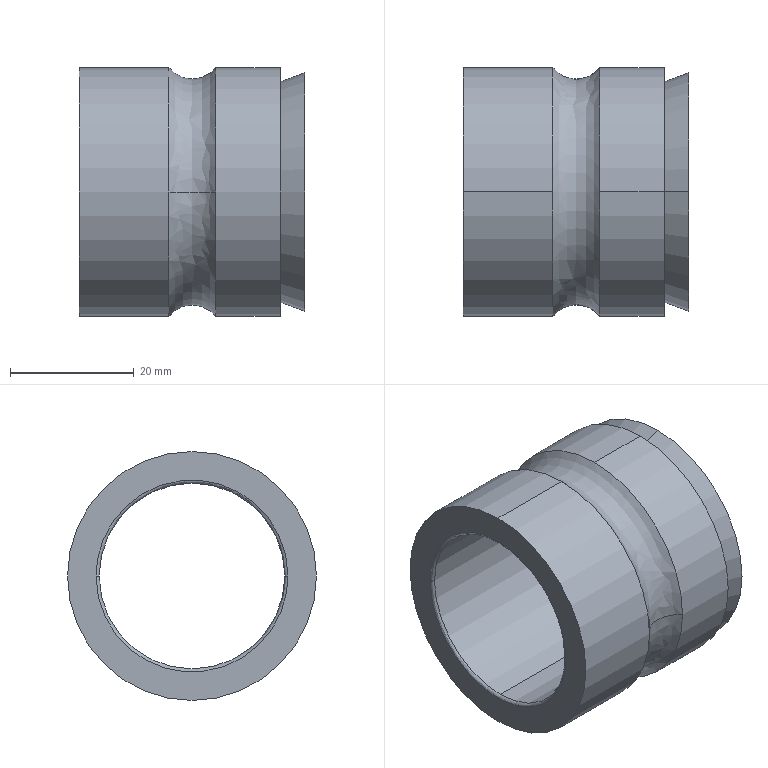Part | SolidWorks | features BaseBody 1 | 1 solid | 17 faces | box 36.5 x 40.2 x 40.2 mm | volume 18564 mm3 | spline 6 | cylinder 6 | plane 3 | cone 2 | commonest cylinder face diameters 40.2 x4 30 x2
STEP:
#1=CARTESIAN_POINT('',(17.7,48.,42.9));
#2=VERTEX_POINT('',#1);
#3=CARTESIAN_POINT('',(17.7,63.,27.9));
#4=VERTEX_POINT('',#3);
#5=CARTESIAN_POINT('',(17.7,63.,42.9));
#6=DIRECTION('',(1.,0.,0.));
#7=DIRECTION('',(0.,0.,1.));
#8=AXIS2_PLACEMENT_3D('',#5,#6,#7);
#9=CIRCLE('',#8,15.);
#10=EDGE_CURVE('',#2,#4,#9,.T.);
#11=ORIENTED_EDGE('',*,*,#10,.F.);
#12=CARTESIAN_POINT('',(18.2,47.5,42.9));
#13=VERTEX_POINT('',#12);
#14=CARTESIAN_POINT('',(17.7,47.5,42.9));
#15=DIRECTION('',(0.,0.,-1.));
#16=DIRECTION('',(0.,-1.,0.));
#17=AXIS2_PLACEMENT_3D('',#14,#15,#16);
#18=CIRCLE('',#17,0.5);
#19=EDGE_CURVE('',#2,#13,#18,.T.);
#20=ORIENTED_EDGE('',*,*,#19,.T.);
#21=CARTESIAN_POINT('',(18.2,78.5,42.9));
#22=VERTEX_POINT('',#21);
#23=CARTESIAN_POINT('',(18.2,47.5,42.9));
#24=CARTESIAN_POINT('',(18.2,47.5,11.9));
#25=CARTESIAN_POINT('',(18.2,78.5,11.9));
#26=CARTESIAN_POINT('',(18.2,78.5,42.9));
#27=(BOUNDED_CURVE()B_SPLINE_CURVE(3,(#23,#24,#25,#26),.UNSPECIFIED.,.F.,.F.)B_SPLINE_CURVE_WITH_KNOTS((4,4),(0.25,0.75),.UNSPECIFIED.)CURVE()GEOMETRIC_REPRESENTATION_ITEM()RATIONAL_B_SPLINE_CURVE((1.,0.3333,0.3333,1.))REPRESENTATION_ITEM(''));
#28=EDGE_CURVE('',#13,#22,#27,.T.);
#29=ORIENTED_EDGE('',*,*,#28,.T.);
#30=CARTESIAN_POINT('',(17.7,78.,42.9));
#31=VERTEX_POINT('',#30);
#32=CARTESIAN_POINT('',(17.7,78.5,42.9));
#33=DIRECTION('',(0.,0.,1.));
#34=DIRECTION('',(0.,1.,0.));
#35=AXIS2_PLACEMENT_3D('',#32,#33,#34);
#36=CIRCLE('',#35,0.5);
#37=EDGE_CURVE('',#31,#22,#36,.T.);
#38=ORIENTED_EDGE('',*,*,#37,.F.);
#39=CARTESIAN_POINT('',(17.7,63.,42.9));
#40=DIRECTION('',(1.,0.,0.));
#41=DIRECTION('',(0.,0.,1.));
#42=AXIS2_PLACEMENT_3D('',#39,#40,#41);
#43=CIRCLE('',#42,15.);
#44=EDGE_CURVE('',#4,#31,#43,.T.);
#45=ORIENTED_EDGE('',*,*,#44,.F.);
#46=EDGE_LOOP('',(#11,#20,#29,#38,#45));
#47=FACE_OUTER_BOUND('',#46,.T.);
#48=CARTESIAN_POINT('',(17.7,48.,42.9));
#49=CARTESIAN_POINT('',(17.7,48.,12.9));
#50=CARTESIAN_POINT('',(17.7,78.,12.9));
#51=CARTESIAN_POINT('',(17.7,78.,42.9));
#52=CARTESIAN_POINT('',(17.993,48.,42.9));
#53=CARTESIAN_POINT('',(17.993,48.,12.9));
#54=CARTESIAN_POINT('',(17.993,78.,12.9));
#55=CARTESIAN_POINT('',(17.993,78.,42.9));
#56=CARTESIAN_POINT('',(18.2,47.793,42.9));
#57=CARTESIAN_POINT('',(18.2,47.793,12.486));
#58=CARTESIAN_POINT('',(18.2,78.207,12.486));
#59=CARTESIAN_POINT('',(18.2,78.207,42.9));
#60=CARTESIAN_POINT('',(18.2,47.5,42.9));
#61=CARTESIAN_POINT('',(18.2,47.5,11.9));
#62=CARTESIAN_POINT('',(18.2,78.5,11.9));
#63=CARTESIAN_POINT('',(18.2,78.5,42.9));
#64=(BOUNDED_SURFACE()B_SPLINE_SURFACE(3,3,((#48,#49,#50,#51),(#52,#53,#54,#55),(#56,#57,#58,#59),(#60,#61,#62,#63)),.UNSPECIFIED.,.F.,.F.,.F.)B_SPLINE_SURFACE_WITH_KNOTS((4,4),(4,4),(0.,1.),(0.,1.),.UNSPECIFIED.)GEOMETRIC_REPRESENTATION_ITEM()RATIONAL_B_SPLINE_SURFACE(((1.,0.3333,0.3333,1.),(0.8047,0.2682,0.2682,0.8047),(0.8047,0.2682,0.2682,0.8047),(1.,0.3333,0.3333,1.)))REPRESENTATION_ITEM('')SURFACE());
#65=ADVANCED_FACE('',(#47),#64,.T.);
#66=CARTESIAN_POINT('',(-18.3,78.5,42.9));
#67=VERTEX_POINT('',#66);
#68=CARTESIAN_POINT('',(-18.3,47.5,42.9));
#69=VERTEX_POINT('',#68);
#70=CARTESIAN_POINT('',(-18.3,78.5,42.9));
#71=CARTESIAN_POINT('',(-18.3,78.5,11.9));
#72=CARTESIAN_POINT('',(-18.3,47.5,11.9));
#73=CARTESIAN_POINT('',(-18.3,47.5,42.9));
#74=(BOUNDED_CURVE()B_SPLINE_CURVE(3,(#70,#71,#72,#73),.UNSPECIFIED.,.F.,.F.)B_SPLINE_CURVE_WITH_KNOTS((4,4),(0.25,0.75),.UNSPECIFIED.)CURVE()GEOMETRIC_REPRESENTATION_ITEM()RATIONAL_B_SPLINE_CURVE((1.,0.3333,0.3333,1.))REPRESENTATION_ITEM(''));
#75=EDGE_CURVE('',#67,#69,#74,.T.);
#76=ORIENTED_EDGE('',*,*,#75,.T.);
#77=CARTESIAN_POINT('',(-17.8,48.,42.9));
#78=VERTEX_POINT('',#77);
#79=CARTESIAN_POINT('',(-17.8,47.5,42.9));
#80=DIRECTION('',(0.,0.,-1.));
#81=DIRECTION('',(0.,-1.,0.));
#82=AXIS2_PLACEMENT_3D('',#79,#80,#81);
#83=CIRCLE('',#82,0.5);
#84=EDGE_CURVE('',#69,#78,#83,.T.);
#85=ORIENTED_EDGE('',*,*,#84,.T.);
#86=CARTESIAN_POINT('',(-17.8,63.,27.9));
#87=VERTEX_POINT('',#86);
#88=CARTESIAN_POINT('',(-17.8,63.,42.9));
#89=DIRECTION('',(-1.,0.,0.));
#90=DIRECTION('',(0.,0.,1.));
#91=AXIS2_PLACEMENT_3D('',#88,#89,#90);
#92=CIRCLE('',#91,15.);
#93=EDGE_CURVE('',#87,#78,#92,.T.);
#94=ORIENTED_EDGE('',*,*,#93,.F.);
#95=CARTESIAN_POINT('',(-17.8,78.,42.9));
#96=VERTEX_POINT('',#95);
#97=CARTESIAN_POINT('',(-17.8,63.,42.9));
#98=DIRECTION('',(-1.,0.,0.));
#99=DIRECTION('',(0.,0.,1.));
#100=AXIS2_PLACEMENT_3D('',#97,#98,#99);
#101=CIRCLE('',#100,15.);
#102=EDGE_CURVE('',#96,#87,#101,.T.);
#103=ORIENTED_EDGE('',*,*,#102,.F.);
#104=CARTESIAN_POINT('',(-17.8,78.5,42.9));
#105=DIRECTION('',(0.,0.,1.));
#106=DIRECTION('',(0.,1.,0.));
#107=AXIS2_PLACEMENT_3D('',#104,#105,#106);
#108=CIRCLE('',#107,0.5);
#109=EDGE_CURVE('',#67,#96,#108,.T.);
#110=ORIENTED_EDGE('',*,*,#109,.F.);
#111=EDGE_LOOP('',(#76,#85,#94,#103,#110));
#112=FACE_OUTER_BOUND('',#111,.T.);
#113=CARTESIAN_POINT('',(-18.3,47.5,42.9));
#114=CARTESIAN_POINT('',(-18.3,47.5,11.9));
#115=CARTESIAN_POINT('',(-18.3,78.5,11.9));
#116=CARTESIAN_POINT('',(-18.3,78.5,42.9));
#117=CARTESIAN_POINT('',(-18.3,47.793,42.9));
#118=CARTESIAN_POINT('',(-18.3,47.793,12.486));
#119=CARTESIAN_POINT('',(-18.3,78.207,12.486));
#120=CARTESIAN_POINT('',(-18.3,78.207,42.9));
#121=CARTESIAN_POINT('',(-18.093,48.,42.9));
#122=CARTESIAN_POINT('',(-18.093,48.,12.9));
#123=CARTESIAN_POINT('',(-18.093,78.,12.9));
#124=CARTESIAN_POINT('',(-18.093,78.,42.9));
#125=CARTESIAN_POINT('',(-17.8,48.,42.9));
#126=CARTESIAN_POINT('',(-17.8,48.,12.9));
#127=CARTESIAN_POINT('',(-17.8,78.,12.9));
#128=CARTESIAN_POINT('',(-17.8,78.,42.9));
#129=(BOUNDED_SURFACE()B_SPLINE_SURFACE(3,3,((#113,#114,#115,#116),(#117,#118,#119,#120),(#121,#122,#123,#124),(#125,#126,#127,#128)),.UNSPECIFIED.,.F.,.F.,.F.)B_SPLINE_SURFACE_WITH_KNOTS((4,4),(4,4),(0.,1.),(0.,1.),.UNSPECIFIED.)GEOMETRIC_REPRESENTATION_ITEM()RATIONAL_B_SPLINE_SURFACE(((1.,0.3333,0.3333,1.),(0.8047,0.2682,0.2682,0.8047),(0.8047,0.2682,0.2682,0.8047),(1.,0.3333,0.3333,1.)))REPRESENTATION_ITEM('')SURFACE());
#130=ADVANCED_FACE('',(#112),#129,.T.);
#131=CARTESIAN_POINT('',(3.778,63.,22.8));
#132=VERTEX_POINT('',#131);
#133=CARTESIAN_POINT('',(3.778,42.9,42.9));
#134=VERTEX_POINT('',#133);
#135=CARTESIAN_POINT('',(3.778,63.,42.9));
#136=DIRECTION('',(-1.,0.,0.));
#137=DIRECTION('',(0.,1.,0.));
#138=AXIS2_PLACEMENT_3D('',#135,#136,#137);
#139=CIRCLE('',#138,20.1);
#140=EDGE_CURVE('',#132,#134,#139,.T.);
#141=ORIENTED_EDGE('',*,*,#140,.T.);
#142=CARTESIAN_POINT('',(-3.778,42.9,42.9));
#143=VERTEX_POINT('',#142);
#144=CARTESIAN_POINT('',(0.,40.,42.9));
#145=DIRECTION('',(0.,0.,1.));
#146=DIRECTION('',(0.,-1.,0.));
#147=AXIS2_PLACEMENT_3D('',#144,#145,#146);
#148=CIRCLE('',#147,4.762);
#149=EDGE_CURVE('',#134,#143,#148,.T.);
#150=ORIENTED_EDGE('',*,*,#149,.T.);
#151=CARTESIAN_POINT('',(-3.778,63.,22.8));
#152=VERTEX_POINT('',#151);
#153=CARTESIAN_POINT('',(-3.778,63.,42.9));
#154=DIRECTION('',(-1.,0.,0.));
#155=DIRECTION('',(0.,0.,-1.));
#156=AXIS2_PLACEMENT_3D('',#153,#154,#155);
#157=CIRCLE('',#156,20.1);
#158=EDGE_CURVE('',#152,#143,#157,.T.);
#159=ORIENTED_EDGE('',*,*,#158,.F.);
#160=CARTESIAN_POINT('',(-3.778,83.1,42.9));
#161=VERTEX_POINT('',#160);
#162=CARTESIAN_POINT('',(-3.778,63.,42.9));
#163=DIRECTION('',(-1.,0.,0.));
#164=DIRECTION('',(0.,0.,-1.));
#165=AXIS2_PLACEMENT_3D('',#162,#163,#164);
#166=CIRCLE('',#165,20.1);
#167=EDGE_CURVE('',#161,#152,#166,.T.);
#168=ORIENTED_EDGE('',*,*,#167,.F.);
#169=CARTESIAN_POINT('',(3.778,83.1,42.9));
#170=VERTEX_POINT('',#169);
#171=CARTESIAN_POINT('',(0.,86.,42.9));
#172=DIRECTION('',(0.,0.,-1.));
#173=DIRECTION('',(0.,1.,0.));
#174=AXIS2_PLACEMENT_3D('',#171,#172,#173);
#175=CIRCLE('',#174,4.763);
#176=EDGE_CURVE('',#170,#161,#175,.T.);
#177=ORIENTED_EDGE('',*,*,#176,.F.);
#178=CARTESIAN_POINT('',(3.778,63.,42.9));
#179=DIRECTION('',(-1.,0.,0.));
#180=DIRECTION('',(0.,1.,0.));
#181=AXIS2_PLACEMENT_3D('',#178,#179,#180);
#182=CIRCLE('',#181,20.1);
#183=EDGE_CURVE('',#170,#132,#182,.T.);
#184=ORIENTED_EDGE('',*,*,#183,.T.);
#185=EDGE_LOOP('',(#141,#150,#159,#168,#177,#184));
#186=FACE_OUTER_BOUND('',#185,.T.);
#187=CARTESIAN_POINT('',(3.778,42.9,42.9));
#188=CARTESIAN_POINT('',(3.778,42.9,2.7));
#189=CARTESIAN_POINT('',(3.778,83.1,2.7));
#190=CARTESIAN_POINT('',(3.778,83.1,42.9));
#191=CARTESIAN_POINT('',(1.703,45.602,42.9));
#192=CARTESIAN_POINT('',(1.703,45.602,8.105));
#193=CARTESIAN_POINT('',(1.703,80.398,8.105));
#194=CARTESIAN_POINT('',(1.703,80.398,42.9));
#195=CARTESIAN_POINT('',(-1.703,45.602,42.9));
#196=CARTESIAN_POINT('',(-1.703,45.602,8.105));
#197=CARTESIAN_POINT('',(-1.703,80.398,8.105));
#198=CARTESIAN_POINT('',(-1.703,80.398,42.9));
#199=CARTESIAN_POINT('',(-3.778,42.9,42.9));
#200=CARTESIAN_POINT('',(-3.778,42.9,2.7));
#201=CARTESIAN_POINT('',(-3.778,83.1,2.7));
#202=CARTESIAN_POINT('',(-3.778,83.1,42.9));
#203=(BOUNDED_SURFACE()B_SPLINE_SURFACE(3,3,((#187,#188,#189,#190),(#191,#192,#193,#194),(#195,#196,#197,#198),(#199,#200,#201,#202)),.UNSPECIFIED.,.F.,.F.,.F.)B_SPLINE_SURFACE_WITH_KNOTS((4,4),(4,4),(0.,1.),(0.,1.),.UNSPECIFIED.)GEOMETRIC_REPRESENTATION_ITEM()RATIONAL_B_SPLINE_SURFACE(((1.,0.3333,0.3333,1.),(0.7393,0.2464,0.2464,0.7393),(0.7393,0.2464,0.2464,0.7393),(1.,0.3333,0.3333,1.)))REPRESENTATION_ITEM('')SURFACE());
#204=ADVANCED_FACE('',(#186),#203,.T.);
#205=ORIENTED_EDGE('',*,*,#93,.T.);
#206=CARTESIAN_POINT('',(-17.8,63.,57.9));
#207=VERTEX_POINT('',#206);
#208=CARTESIAN_POINT('',(-17.8,63.,42.9));
#209=DIRECTION('',(-1.,0.,0.));
#210=DIRECTION('',(0.,0.,1.));
#211=AXIS2_PLACEMENT_3D('',#208,#209,#210);
#212=CIRCLE('',#211,15.);
#213=EDGE_CURVE('',#78,#207,#212,.T.);
#214=ORIENTED_EDGE('',*,*,#213,.T.);
#215=CARTESIAN_POINT('',(17.7,63.,57.9));
#216=VERTEX_POINT('',#215);
#217=CARTESIAN_POINT('',(-17.8,63.,57.9));
#218=DIRECTION('',(1.,0.,0.));
#219=VECTOR('',#218,1000.);
#220=LINE('',#217,#219);
#221=EDGE_CURVE('',#207,#216,#220,.T.);
#222=ORIENTED_EDGE('',*,*,#221,.T.);
#223=CARTESIAN_POINT('',(17.7,63.,42.9));
#224=DIRECTION('',(1.,0.,0.));
#225=DIRECTION('',(0.,0.,1.));
#226=AXIS2_PLACEMENT_3D('',#223,#224,#225);
#227=CIRCLE('',#226,15.);
#228=EDGE_CURVE('',#216,#2,#227,.T.);
#229=ORIENTED_EDGE('',*,*,#228,.T.);
#230=ORIENTED_EDGE('',*,*,#10,.T.);
#231=CARTESIAN_POINT('',(-17.8,63.,27.9));
#232=DIRECTION('',(1.,0.,0.));
#233=VECTOR('',#232,1000.);
#234=LINE('',#231,#233);
#235=EDGE_CURVE('',#87,#4,#234,.T.);
#236=ORIENTED_EDGE('',*,*,#235,.F.);
#237=EDGE_LOOP('',(#205,#214,#222,#229,#230,#236));
#238=FACE_OUTER_BOUND('',#237,.T.);
#239=CARTESIAN_POINT('',(-17.8,63.,42.9));
#240=DIRECTION('',(1.,0.,0.));
#241=DIRECTION('',(0.,0.,-1.));
#242=AXIS2_PLACEMENT_3D('',#239,#240,#241);
#243=CYLINDRICAL_SURFACE('',#242,15.);
#244=ADVANCED_FACE('',(#238),#243,.F.);
#245=CARTESIAN_POINT('',(14.2,63.,25.1));
#246=VERTEX_POINT('',#245);
#247=CARTESIAN_POINT('',(14.2,63.,60.7));
#248=VERTEX_POINT('',#247);
#249=CARTESIAN_POINT('',(14.2,63.,42.9));
#250=DIRECTION('',(1.,0.,0.));
#251=DIRECTION('',(0.,0.,-1.));
#252=AXIS2_PLACEMENT_3D('',#249,#250,#251);
#253=CIRCLE('',#252,17.8);
#254=EDGE_CURVE('',#246,#248,#253,.T.);
#255=ORIENTED_EDGE('',*,*,#254,.T.);
#256=CARTESIAN_POINT('',(18.2,63.,62.156));
#257=VERTEX_POINT('',#256);
#258=CARTESIAN_POINT('',(18.2,63.,62.156));
#259=DIRECTION('',(0.9397,0.,0.342));
#260=VECTOR('',#259,1000.);
#261=LINE('',#258,#260);
#262=EDGE_CURVE('',#248,#257,#261,.T.);
#263=ORIENTED_EDGE('',*,*,#262,.T.);
#264=CARTESIAN_POINT('',(18.2,63.,23.644));
#265=VERTEX_POINT('',#264);
#266=CARTESIAN_POINT('',(18.2,63.,42.9));
#267=DIRECTION('',(1.,0.,0.));
#268=DIRECTION('',(0.,0.,-1.));
#269=AXIS2_PLACEMENT_3D('',#266,#267,#268);
#270=CIRCLE('',#269,19.256);
#271=EDGE_CURVE('',#265,#257,#270,.T.);
#272=ORIENTED_EDGE('',*,*,#271,.F.);
#273=CARTESIAN_POINT('',(18.2,63.,23.644));
#274=DIRECTION('',(0.9397,0.,-0.342));
#275=VECTOR('',#274,1000.);
#276=LINE('',#273,#275);
#277=EDGE_CURVE('',#246,#265,#276,.T.);
#278=ORIENTED_EDGE('',*,*,#277,.F.);
#279=EDGE_LOOP('',(#255,#263,#272,#278));
#280=FACE_OUTER_BOUND('',#279,.T.);
#281=CARTESIAN_POINT('',(18.2,63.,42.9));
#282=DIRECTION('',(1.,0.,0.));
#283=DIRECTION('',(0.,0.,-1.));
#284=AXIS2_PLACEMENT_3D('',#281,#282,#283);
#285=CONICAL_SURFACE('',#284,19.256,0.3491);
#286=ADVANCED_FACE('',(#280),#285,.T.);
#287=CARTESIAN_POINT('',(-18.3,63.,63.));
#288=VERTEX_POINT('',#287);
#289=CARTESIAN_POINT('',(-18.3,63.,22.8));
#290=VERTEX_POINT('',#289);
#291=CARTESIAN_POINT('',(-18.3,63.,42.9));
#292=DIRECTION('',(-1.,0.,0.));
#293=DIRECTION('',(0.,0.,-1.));
#294=AXIS2_PLACEMENT_3D('',#291,#292,#293);
#295=CIRCLE('',#294,20.1);
#296=EDGE_CURVE('',#288,#290,#295,.T.);
#297=ORIENTED_EDGE('',*,*,#296,.F.);
#298=CARTESIAN_POINT('',(-3.778,63.,63.));
#299=VERTEX_POINT('',#298);
#300=CARTESIAN_POINT('',(-11.039,63.,63.));
#301=DIRECTION('',(1.,0.,0.));
#302=VECTOR('',#301,1000.);
#303=LINE('',#300,#302);
#304=EDGE_CURVE('',#288,#299,#303,.T.);
#305=ORIENTED_EDGE('',*,*,#304,.T.);
#306=CARTESIAN_POINT('',(-3.778,63.,42.9));
#307=DIRECTION('',(-1.,0.,0.));
#308=DIRECTION('',(0.,0.,-1.));
#309=AXIS2_PLACEMENT_3D('',#306,#307,#308);
#310=CIRCLE('',#309,20.1);
#311=EDGE_CURVE('',#299,#161,#310,.T.);
#312=ORIENTED_EDGE('',*,*,#311,.T.);
#313=ORIENTED_EDGE('',*,*,#167,.T.);
#314=CARTESIAN_POINT('',(-11.039,63.,22.8));
#315=DIRECTION('',(1.,0.,0.));
#316=VECTOR('',#315,1000.);
#317=LINE('',#314,#316);
#318=EDGE_CURVE('',#290,#152,#317,.T.);
#319=ORIENTED_EDGE('',*,*,#318,.F.);
#320=EDGE_LOOP('',(#297,#305,#312,#313,#319));
#321=FACE_OUTER_BOUND('',#320,.T.);
#322=CARTESIAN_POINT('',(-11.039,63.,42.9));
#323=DIRECTION('',(1.,0.,0.));
#324=DIRECTION('',(0.,0.,-1.));
#325=AXIS2_PLACEMENT_3D('',#322,#323,#324);
#326=CYLINDRICAL_SURFACE('',#325,20.1);
#327=ADVANCED_FACE('',(#321),#326,.T.);
#328=CARTESIAN_POINT('',(3.778,63.,63.));
#329=VERTEX_POINT('',#328);
#330=CARTESIAN_POINT('',(3.778,63.,42.9));
#331=DIRECTION('',(-1.,0.,0.));
#332=DIRECTION('',(0.,1.,0.));
#333=AXIS2_PLACEMENT_3D('',#330,#331,#332);
#334=CIRCLE('',#333,20.1);
#335=EDGE_CURVE('',#329,#170,#334,.T.);
#336=ORIENTED_EDGE('',*,*,#335,.F.);
#337=CARTESIAN_POINT('',(14.2,63.,63.));
#338=VERTEX_POINT('',#337);
#339=CARTESIAN_POINT('',(8.989,63.,63.));
#340=DIRECTION('',(1.,0.,0.));
#341=VECTOR('',#340,1000.);
#342=LINE('',#339,#341);
#343=EDGE_CURVE('',#329,#338,#342,.T.);
#344=ORIENTED_EDGE('',*,*,#343,.T.);
#345=CARTESIAN_POINT('',(14.2,63.,22.8));
#346=VERTEX_POINT('',#345);
#347=CARTESIAN_POINT('',(14.2,63.,42.9));
#348=DIRECTION('',(1.,0.,0.));
#349=DIRECTION('',(0.,0.,-1.));
#350=AXIS2_PLACEMENT_3D('',#347,#348,#349);
#351=CIRCLE('',#350,20.1);
#352=EDGE_CURVE('',#346,#338,#351,.T.);
#353=ORIENTED_EDGE('',*,*,#352,.F.);
#354=CARTESIAN_POINT('',(8.989,63.,22.8));
#355=DIRECTION('',(1.,0.,0.));
#356=VECTOR('',#355,1000.);
#357=LINE('',#354,#356);
#358=EDGE_CURVE('',#132,#346,#357,.T.);
#359=ORIENTED_EDGE('',*,*,#358,.F.);
#360=ORIENTED_EDGE('',*,*,#183,.F.);
#361=EDGE_LOOP('',(#336,#344,#353,#359,#360));
#362=FACE_OUTER_BOUND('',#361,.T.);
#363=CARTESIAN_POINT('',(8.989,63.,42.9));
#364=DIRECTION('',(1.,0.,0.));
#365=DIRECTION('',(0.,0.,-1.));
#366=AXIS2_PLACEMENT_3D('',#363,#364,#365);
#367=CYLINDRICAL_SURFACE('',#366,20.1);
#368=ADVANCED_FACE('',(#362),#367,.T.);
#369=ORIENTED_EDGE('',*,*,#221,.F.);
#370=CARTESIAN_POINT('',(-17.8,63.,42.9));
#371=DIRECTION('',(-1.,0.,0.));
#372=DIRECTION('',(0.,0.,1.));
#373=AXIS2_PLACEMENT_3D('',#370,#371,#372);
#374=CIRCLE('',#373,15.);
#375=EDGE_CURVE('',#207,#96,#374,.T.);
#376=ORIENTED_EDGE('',*,*,#375,.T.);
#377=ORIENTED_EDGE('',*,*,#102,.T.);
#378=ORIENTED_EDGE('',*,*,#235,.T.);
#379=ORIENTED_EDGE('',*,*,#44,.T.);
#380=CARTESIAN_POINT('',(17.7,63.,42.9));
#381=DIRECTION('',(1.,0.,0.));
#382=DIRECTION('',(0.,0.,1.));
#383=AXIS2_PLACEMENT_3D('',#380,#381,#382);
#384=CIRCLE('',#383,15.);
#385=EDGE_CURVE('',#31,#216,#384,.T.);
#386=ORIENTED_EDGE('',*,*,#385,.T.);
#387=EDGE_LOOP('',(#369,#376,#377,#378,#379,#386));
#388=FACE_OUTER_BOUND('',#387,.T.);
#389=CARTESIAN_POINT('',(-17.8,63.,42.9));
#390=DIRECTION('',(1.,0.,0.));
#391=DIRECTION('',(0.,0.,-1.));
#392=AXIS2_PLACEMENT_3D('',#389,#390,#391);
#393=CYLINDRICAL_SURFACE('',#392,15.);
#394=ADVANCED_FACE('',(#388),#393,.F.);
#395=ORIENTED_EDGE('',*,*,#19,.F.);
#396=ORIENTED_EDGE('',*,*,#228,.F.);
#397=ORIENTED_EDGE('',*,*,#385,.F.);
#398=ORIENTED_EDGE('',*,*,#37,.T.);
#399=CARTESIAN_POINT('',(18.2,78.5,42.9));
#400=CARTESIAN_POINT('',(18.2,78.5,73.9));
#401=CARTESIAN_POINT('',(18.2,47.5,73.9));
#402=CARTESIAN_POINT('',(18.2,47.5,42.9));
#403=(BOUNDED_CURVE()B_SPLINE_CURVE(3,(#399,#400,#401,#402),.UNSPECIFIED.,.F.,.F.)B_SPLINE_CURVE_WITH_KNOTS((4,4),(0.75,1.25),.UNSPECIFIED.)CURVE()GEOMETRIC_REPRESENTATION_ITEM()RATIONAL_B_SPLINE_CURVE((1.,0.3333,0.3333,1.))REPRESENTATION_ITEM(''));
#404=EDGE_CURVE('',#22,#13,#403,.T.);
#405=ORIENTED_EDGE('',*,*,#404,.T.);
#406=EDGE_LOOP('',(#395,#396,#397,#398,#405));
#407=FACE_OUTER_BOUND('',#406,.T.);
#408=CARTESIAN_POINT('',(17.7,78.,42.9));
#409=CARTESIAN_POINT('',(17.7,78.,72.9));
#410=CARTESIAN_POINT('',(17.7,48.,72.9));
#411=CARTESIAN_POINT('',(17.7,48.,42.9));
#412=CARTESIAN_POINT('',(17.993,78.,42.9));
#413=CARTESIAN_POINT('',(17.993,78.,72.9));
#414=CARTESIAN_POINT('',(17.993,48.,72.9));
#415=CARTESIAN_POINT('',(17.993,48.,42.9));
#416=CARTESIAN_POINT('',(18.2,78.207,42.9));
#417=CARTESIAN_POINT('',(18.2,78.207,73.314));
#418=CARTESIAN_POINT('',(18.2,47.793,73.314));
#419=CARTESIAN_POINT('',(18.2,47.793,42.9));
#420=CARTESIAN_POINT('',(18.2,78.5,42.9));
#421=CARTESIAN_POINT('',(18.2,78.5,73.9));
#422=CARTESIAN_POINT('',(18.2,47.5,73.9));
#423=CARTESIAN_POINT('',(18.2,47.5,42.9));
#424=(BOUNDED_SURFACE()B_SPLINE_SURFACE(3,3,((#408,#409,#410,#411),(#412,#413,#414,#415),(#416,#417,#418,#419),(#420,#421,#422,#423)),.UNSPECIFIED.,.F.,.F.,.F.)B_SPLINE_SURFACE_WITH_KNOTS((4,4),(4,4),(0.,1.),(0.,1.),.UNSPECIFIED.)GEOMETRIC_REPRESENTATION_ITEM()RATIONAL_B_SPLINE_SURFACE(((1.,0.3333,0.3333,1.),(0.8047,0.2682,0.2682,0.8047),(0.8047,0.2682,0.2682,0.8047),(1.,0.3333,0.3333,1.)))REPRESENTATION_ITEM('')SURFACE());
#425=ADVANCED_FACE('',(#407),#424,.T.);
#426=ORIENTED_EDGE('',*,*,#84,.F.);
#427=CARTESIAN_POINT('',(-18.3,47.5,42.9));
#428=CARTESIAN_POINT('',(-18.3,47.5,73.9));
#429=CARTESIAN_POINT('',(-18.3,78.5,73.9));
#430=CARTESIAN_POINT('',(-18.3,78.5,42.9));
#431=(BOUNDED_CURVE()B_SPLINE_CURVE(3,(#427,#428,#429,#430),.UNSPECIFIED.,.F.,.F.)B_SPLINE_CURVE_WITH_KNOTS((4,4),(0.75,1.25),.UNSPECIFIED.)CURVE()GEOMETRIC_REPRESENTATION_ITEM()RATIONAL_B_SPLINE_CURVE((1.,0.3333,0.3333,1.))REPRESENTATION_ITEM(''));
#432=EDGE_CURVE('',#69,#67,#431,.T.);
#433=ORIENTED_EDGE('',*,*,#432,.T.);
#434=ORIENTED_EDGE('',*,*,#109,.T.);
#435=ORIENTED_EDGE('',*,*,#375,.F.);
#436=ORIENTED_EDGE('',*,*,#213,.F.);
#437=EDGE_LOOP('',(#426,#433,#434,#435,#436));
#438=FACE_OUTER_BOUND('',#437,.T.);
#439=CARTESIAN_POINT('',(-18.3,78.5,42.9));
#440=CARTESIAN_POINT('',(-18.3,78.5,73.9));
#441=CARTESIAN_POINT('',(-18.3,47.5,73.9));
#442=CARTESIAN_POINT('',(-18.3,47.5,42.9));
#443=CARTESIAN_POINT('',(-18.3,78.207,42.9));
#444=CARTESIAN_POINT('',(-18.3,78.207,73.314));
#445=CARTESIAN_POINT('',(-18.3,47.793,73.314));
#446=CARTESIAN_POINT('',(-18.3,47.793,42.9));
#447=CARTESIAN_POINT('',(-18.093,78.,42.9));
#448=CARTESIAN_POINT('',(-18.093,78.,72.9));
#449=CARTESIAN_POINT('',(-18.093,48.,72.9));
#450=CARTESIAN_POINT('',(-18.093,48.,42.9));
#451=CARTESIAN_POINT('',(-17.8,78.,42.9));
#452=CARTESIAN_POINT('',(-17.8,78.,72.9));
#453=CARTESIAN_POINT('',(-17.8,48.,72.9));
#454=CARTESIAN_POINT('',(-17.8,48.,42.9));
#455=(BOUNDED_SURFACE()B_SPLINE_SURFACE(3,3,((#439,#440,#441,#442),(#443,#444,#445,#446),(#447,#448,#449,#450),(#451,#452,#453,#454)),.UNSPECIFIED.,.F.,.F.,.F.)B_SPLINE_SURFACE_WITH_KNOTS((4,4),(4,4),(0.,1.),(0.,1.),.UNSPECIFIED.)GEOMETRIC_REPRESENTATION_ITEM()RATIONAL_B_SPLINE_SURFACE(((1.,0.3333,0.3333,1.),(0.8047,0.2682,0.2682,0.8047),(0.8047,0.2682,0.2682,0.8047),(1.,0.3333,0.3333,1.)))REPRESENTATION_ITEM('')SURFACE());
#456=ADVANCED_FACE('',(#438),#455,.T.);
#457=ORIENTED_EDGE('',*,*,#271,.T.);
#458=CARTESIAN_POINT('',(18.2,63.,42.9));
#459=DIRECTION('',(1.,0.,0.));
#460=DIRECTION('',(0.,0.,-1.));
#461=AXIS2_PLACEMENT_3D('',#458,#459,#460);
#462=CIRCLE('',#461,19.256);
#463=EDGE_CURVE('',#257,#265,#462,.T.);
#464=ORIENTED_EDGE('',*,*,#463,.T.);
#465=EDGE_LOOP('',(#457,#464));
#466=FACE_OUTER_BOUND('',#465,.T.);
#467=ORIENTED_EDGE('',*,*,#404,.F.);
#468=ORIENTED_EDGE('',*,*,#28,.F.);
#469=EDGE_LOOP('',(#467,#468));
#470=FACE_BOUND('',#469,.T.);
#471=CARTESIAN_POINT('',(18.2,63.,60.278));
#472=DIRECTION('',(1.,0.,0.));
#473=DIRECTION('',(0.,0.,-1.));
#474=AXIS2_PLACEMENT_3D('',#471,#472,#473);
#475=PLANE('',#474);
#476=ADVANCED_FACE('',(#466,#470),#475,.T.);
#477=ORIENTED_EDGE('',*,*,#75,.F.);
#478=ORIENTED_EDGE('',*,*,#432,.F.);
#479=EDGE_LOOP('',(#477,#478));
#480=FACE_BOUND('',#479,.T.);
#481=CARTESIAN_POINT('',(-18.3,63.,42.9));
#482=DIRECTION('',(-1.,0.,0.));
#483=DIRECTION('',(0.,0.,-1.));
#484=AXIS2_PLACEMENT_3D('',#481,#482,#483);
#485=CIRCLE('',#484,20.1);
#486=EDGE_CURVE('',#290,#288,#485,.T.);
#487=ORIENTED_EDGE('',*,*,#486,.T.);
#488=ORIENTED_EDGE('',*,*,#296,.T.);
#489=EDGE_LOOP('',(#487,#488));
#490=FACE_OUTER_BOUND('',#489,.T.);
#491=CARTESIAN_POINT('',(-18.3,63.,60.7));
#492=DIRECTION('',(-1.,0.,0.));
#493=DIRECTION('',(0.,0.,1.));
#494=AXIS2_PLACEMENT_3D('',#491,#492,#493);
#495=PLANE('',#494);
#496=ADVANCED_FACE('',(#480,#490),#495,.T.);
#497=ORIENTED_EDGE('',*,*,#262,.F.);
#498=CARTESIAN_POINT('',(14.2,63.,42.9));
#499=DIRECTION('',(1.,0.,0.));
#500=DIRECTION('',(0.,0.,-1.));
#501=AXIS2_PLACEMENT_3D('',#498,#499,#500);
#502=CIRCLE('',#501,17.8);
#503=EDGE_CURVE('',#248,#246,#502,.T.);
#504=ORIENTED_EDGE('',*,*,#503,.T.);
#505=ORIENTED_EDGE('',*,*,#277,.T.);
#506=ORIENTED_EDGE('',*,*,#463,.F.);
#507=EDGE_LOOP('',(#497,#504,#505,#506));
#508=FACE_OUTER_BOUND('',#507,.T.);
#509=CARTESIAN_POINT('',(18.2,63.,42.9));
#510=DIRECTION('',(1.,0.,0.));
#511=DIRECTION('',(0.,0.,-1.));
#512=AXIS2_PLACEMENT_3D('',#509,#510,#511);
#513=CONICAL_SURFACE('',#512,19.256,0.3491);
#514=ADVANCED_FACE('',(#508),#513,.T.);
#515=ORIENTED_EDGE('',*,*,#304,.F.);
#516=ORIENTED_EDGE('',*,*,#486,.F.);
#517=ORIENTED_EDGE('',*,*,#318,.T.);
#518=ORIENTED_EDGE('',*,*,#158,.T.);
#519=CARTESIAN_POINT('',(-3.778,63.,42.9));
#520=DIRECTION('',(-1.,0.,0.));
#521=DIRECTION('',(0.,0.,-1.));
#522=AXIS2_PLACEMENT_3D('',#519,#520,#521);
#523=CIRCLE('',#522,20.1);
#524=EDGE_CURVE('',#143,#299,#523,.T.);
#525=ORIENTED_EDGE('',*,*,#524,.T.);
#526=EDGE_LOOP('',(#515,#516,#517,#518,#525));
#527=FACE_OUTER_BOUND('',#526,.T.);
#528=CARTESIAN_POINT('',(-11.039,63.,42.9));
#529=DIRECTION('',(1.,0.,0.));
#530=DIRECTION('',(0.,0.,-1.));
#531=AXIS2_PLACEMENT_3D('',#528,#529,#530);
#532=CYLINDRICAL_SURFACE('',#531,20.1);
#533=ADVANCED_FACE('',(#527),#532,.T.);
#534=ORIENTED_EDGE('',*,*,#352,.T.);
#535=CARTESIAN_POINT('',(14.2,63.,42.9));
#536=DIRECTION('',(1.,0.,0.));
#537=DIRECTION('',(0.,0.,-1.));
#538=AXIS2_PLACEMENT_3D('',#535,#536,#537);
#539=CIRCLE('',#538,20.1);
#540=EDGE_CURVE('',#338,#346,#539,.T.);
#541=ORIENTED_EDGE('',*,*,#540,.T.);
#542=EDGE_LOOP('',(#534,#541));
#543=FACE_OUTER_BOUND('',#542,.T.);
#544=ORIENTED_EDGE('',*,*,#254,.F.);
#545=ORIENTED_EDGE('',*,*,#503,.F.);
#546=EDGE_LOOP('',(#544,#545));
#547=FACE_BOUND('',#546,.T.);
#548=CARTESIAN_POINT('',(14.2,63.,61.85));
#549=DIRECTION('',(1.,0.,0.));
#550=DIRECTION('',(0.,0.,-1.));
#551=AXIS2_PLACEMENT_3D('',#548,#549,#550);
#552=PLANE('',#551);
#553=ADVANCED_FACE('',(#543,#547),#552,.T.);
#554=ORIENTED_EDGE('',*,*,#149,.F.);
#555=CARTESIAN_POINT('',(3.778,63.,42.9));
#556=DIRECTION('',(-1.,0.,0.));
#557=DIRECTION('',(0.,1.,0.));
#558=AXIS2_PLACEMENT_3D('',#555,#556,#557);
#559=CIRCLE('',#558,20.1);
#560=EDGE_CURVE('',#134,#329,#559,.T.);
#561=ORIENTED_EDGE('',*,*,#560,.T.);
#562=ORIENTED_EDGE('',*,*,#335,.T.);
#563=ORIENTED_EDGE('',*,*,#176,.T.);
#564=ORIENTED_EDGE('',*,*,#311,.F.);
#565=ORIENTED_EDGE('',*,*,#524,.F.);
#566=EDGE_LOOP('',(#554,#561,#562,#563,#564,#565));
#567=FACE_OUTER_BOUND('',#566,.T.);
#568=CARTESIAN_POINT('',(3.778,83.1,42.9));
#569=CARTESIAN_POINT('',(3.778,83.1,83.1));
#570=CARTESIAN_POINT('',(3.778,42.9,83.1));
#571=CARTESIAN_POINT('',(3.778,42.9,42.9));
#572=CARTESIAN_POINT('',(1.703,80.398,42.9));
#573=CARTESIAN_POINT('',(1.703,80.398,77.695));
#574=CARTESIAN_POINT('',(1.703,45.602,77.695));
#575=CARTESIAN_POINT('',(1.703,45.602,42.9));
#576=CARTESIAN_POINT('',(-1.703,80.398,42.9));
#577=CARTESIAN_POINT('',(-1.703,80.398,77.695));
#578=CARTESIAN_POINT('',(-1.703,45.602,77.695));
#579=CARTESIAN_POINT('',(-1.703,45.602,42.9));
#580=CARTESIAN_POINT('',(-3.778,83.1,42.9));
#581=CARTESIAN_POINT('',(-3.778,83.1,83.1));
#582=CARTESIAN_POINT('',(-3.778,42.9,83.1));
#583=CARTESIAN_POINT('',(-3.778,42.9,42.9));
#584=(BOUNDED_SURFACE()B_SPLINE_SURFACE(3,3,((#568,#569,#570,#571),(#572,#573,#574,#575),(#576,#577,#578,#579),(#580,#581,#582,#583)),.UNSPECIFIED.,.F.,.F.,.F.)B_SPLINE_SURFACE_WITH_KNOTS((4,4),(4,4),(0.,1.),(0.,1.),.UNSPECIFIED.)GEOMETRIC_REPRESENTATION_ITEM()RATIONAL_B_SPLINE_SURFACE(((1.,0.3333,0.3333,1.),(0.7393,0.2464,0.2464,0.7393),(0.7393,0.2464,0.2464,0.7393),(1.,0.3333,0.3333,1.)))REPRESENTATION_ITEM('')SURFACE());
#585=ADVANCED_FACE('',(#567),#584,.T.);
#586=ORIENTED_EDGE('',*,*,#343,.F.);
#587=ORIENTED_EDGE('',*,*,#560,.F.);
#588=ORIENTED_EDGE('',*,*,#140,.F.);
#589=ORIENTED_EDGE('',*,*,#358,.T.);
#590=ORIENTED_EDGE('',*,*,#540,.F.);
#591=EDGE_LOOP('',(#586,#587,#588,#589,#590));
#592=FACE_OUTER_BOUND('',#591,.T.);
#593=CARTESIAN_POINT('',(8.989,63.,42.9));
#594=DIRECTION('',(1.,0.,0.));
#595=DIRECTION('',(0.,0.,-1.));
#596=AXIS2_PLACEMENT_3D('',#593,#594,#595);
#597=CYLINDRICAL_SURFACE('',#596,20.1);
#598=ADVANCED_FACE('',(#592),#597,.T.);
#599=CLOSED_SHELL('',(#65,#130,#204,#244,#286,#327,#368,#394,#425,#456,#476,#496,#514,#533,#553,#585,#598));
#600=MANIFOLD_SOLID_BREP('',#599);
#601=CARTESIAN_POINT('',(0.,0.,0.));
#602=DIRECTION('',(0.,0.,1.));
#603=DIRECTION('',(1.,0.,0.));
#604=AXIS2_PLACEMENT_3D('',#601,#602,#603);
#605=(LENGTH_UNIT()NAMED_UNIT(*)SI_UNIT(.MILLI.,.METRE.));
#606=UNCERTAINTY_MEASURE_WITH_UNIT(LENGTH_MEASURE(0.00001),#605,'','');
#607=(NAMED_UNIT(*)PLANE_ANGLE_UNIT()SI_UNIT($,.RADIAN.));
#608=(NAMED_UNIT(*)SI_UNIT($,.STERADIAN.)SOLID_ANGLE_UNIT());
#609=(GEOMETRIC_REPRESENTATION_CONTEXT(3)GLOBAL_UNCERTAINTY_ASSIGNED_CONTEXT((#606))GLOBAL_UNIT_ASSIGNED_CONTEXT((#605,#607,#608))REPRESENTATION_CONTEXT('',''));
#610=ADVANCED_BREP_SHAPE_REPRESENTATION('',(#600,#604),#609);